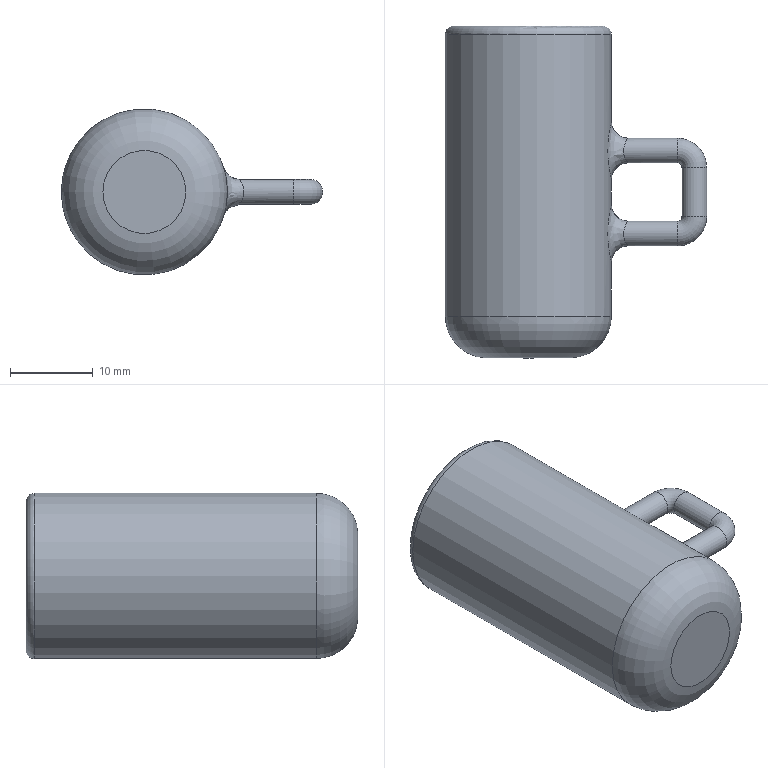Part | NX | features BLEND 4, DATUM_CSYS 2, SWP104 2, REPLACE_FACE 1, SKETCH 1, UNITE 1 | 1 solid | 16 faces | box 31.5 x 40 x 20 mm | volume 6808 mm3 | torus 6 | cylinder 5 | plane 3 | spline 2 | commonest cylinder face diameters 3 x3 14 x1 20 x1
STEP:
#1=CARTESIAN_POINT('',(-10.,5.,0.));
#2=VERTEX_POINT('',#1);
#3=CARTESIAN_POINT('',(0.,5.,0.));
#4=DIRECTION('',(0.,1.,0.));
#5=DIRECTION('',(-1.,0.,0.));
#6=AXIS2_PLACEMENT_3D('',#3,#4,#5);
#7=CIRCLE('',#6,10.);
#8=EDGE_CURVE('',#2,#2,#7,.T.);
#9=ORIENTED_EDGE('',*,*,#8,.T.);
#10=EDGE_LOOP('',(#9));
#11=FACE_BOUND('',#10,.T.);
#12=CARTESIAN_POINT('',(10.,39.,0.));
#13=VERTEX_POINT('',#12);
#14=CARTESIAN_POINT('',(0.,39.,0.));
#15=DIRECTION('',(0.,-1.,0.));
#16=DIRECTION('',(1.,0.,0.));
#17=AXIS2_PLACEMENT_3D('',#14,#15,#16);
#18=CIRCLE('',#17,10.);
#19=EDGE_CURVE('',#13,#13,#18,.T.);
#20=ORIENTED_EDGE('',*,*,#19,.T.);
#21=EDGE_LOOP('',(#20));
#22=FACE_BOUND('',#21,.T.);
#23=CARTESIAN_POINT('',(9.565,15.,2.917));
#24=VERTEX_POINT('',#23);
#25=CARTESIAN_POINT('',(9.699,12.883,2.534));
#26=CARTESIAN_POINT('',(9.475,14.998,3.173));
#27=CARTESIAN_POINT('',(9.7,17.124,2.53));
#28=CARTESIAN_POINT('',(9.942,18.269,1.264));
#29=CARTESIAN_POINT('',(10.029,18.616,0.0008688));
#30=CARTESIAN_POINT('',(9.942,18.269,-1.266));
#31=CARTESIAN_POINT('',(9.7,17.12,-2.532));
#32=CARTESIAN_POINT('',(9.475,15.,-3.173));
#33=CARTESIAN_POINT('',(9.7,12.88,-2.532));
#34=CARTESIAN_POINT('',(9.942,11.73,-1.264));
#35=CARTESIAN_POINT('',(10.029,11.384,0.005302));
#36=CARTESIAN_POINT('',(9.942,11.732,1.267));
#37=CARTESIAN_POINT('',(9.699,12.883,2.534));
#38=CARTESIAN_POINT('',(9.475,14.998,3.173));
#39=CARTESIAN_POINT('',(9.7,17.124,2.53));
#40=B_SPLINE_CURVE_WITH_KNOTS('',3,(#25,#26,#27,#28,#29,#30,#31,#32,#33,#34,#35,#36,#37,#38,#39),.UNSPECIFIED.,.T.,.F.,(1,1,1,1,1,1,1,1,1,1,1,1,1,1,1,1,1,1,1),(-0.005066,-0.003799,-0.002533,0.,0.002533,0.003799,0.005066,0.006332,0.007599,0.01013,0.01266,0.01393,0.0152,0.01646,0.01773,0.02026,0.0228,0.02406,0.02533),.UNSPECIFIED.);
#41=EDGE_CURVE('',#24,#24,#40,.T.);
#42=ORIENTED_EDGE('',*,*,#41,.T.);
#43=EDGE_LOOP('',(#42));
#44=FACE_BOUND('',#43,.T.);
#45=CARTESIAN_POINT('',(9.565,25.,2.917));
#46=VERTEX_POINT('',#45);
#47=CARTESIAN_POINT('',(9.7,22.877,2.531));
#48=CARTESIAN_POINT('',(9.475,25.,3.174));
#49=CARTESIAN_POINT('',(9.7,27.123,2.531));
#50=CARTESIAN_POINT('',(9.942,28.27,1.262));
#51=CARTESIAN_POINT('',(10.029,28.614,0.003138));
#52=CARTESIAN_POINT('',(9.943,28.272,-1.261));
#53=CARTESIAN_POINT('',(9.7,27.122,-2.532));
#54=CARTESIAN_POINT('',(9.475,25.001,-3.173));
#55=CARTESIAN_POINT('',(9.7,22.88,-2.531));
#56=CARTESIAN_POINT('',(9.942,21.732,-1.269));
#57=CARTESIAN_POINT('',(10.029,21.384,0.004067));
#58=CARTESIAN_POINT('',(9.942,21.731,1.263));
#59=CARTESIAN_POINT('',(9.7,22.877,2.531));
#60=CARTESIAN_POINT('',(9.475,25.,3.174));
#61=CARTESIAN_POINT('',(9.7,27.123,2.531));
#62=B_SPLINE_CURVE_WITH_KNOTS('',3,(#47,#48,#49,#50,#51,#52,#53,#54,#55,#56,#57,#58,#59,#60,#61),.UNSPECIFIED.,.T.,.F.,(1,1,1,1,1,1,1,1,1,1,1,1,1,1,1,1,1,1,1),(-0.005105,-0.003829,-0.002552,0.,0.002552,0.003829,0.005105,0.006381,0.007657,0.01021,0.01276,0.01404,0.01531,0.01659,0.01787,0.02042,0.02297,0.02425,0.02552),.UNSPECIFIED.);
#63=EDGE_CURVE('',#46,#46,#62,.T.);
#64=ORIENTED_EDGE('',*,*,#63,.T.);
#65=EDGE_LOOP('',(#64));
#66=FACE_BOUND('',#65,.T.);
#67=CARTESIAN_POINT('',(0.,40.,0.));
#68=DIRECTION('',(0.,-1.,0.));
#69=DIRECTION('',(1.,0.,0.));
#70=AXIS2_PLACEMENT_3D('',#67,#68,#69);
#71=CYLINDRICAL_SURFACE('',#70,10.);
#72=ADVANCED_FACE('',(#11,#22,#44,#66),#71,.T.);
#73=CARTESIAN_POINT('',(2.,2.,0.));
#74=VERTEX_POINT('',#73);
#75=CARTESIAN_POINT('',(0.,2.,0.));
#76=DIRECTION('',(0.,-1.,0.));
#77=DIRECTION('',(1.,0.,0.));
#78=AXIS2_PLACEMENT_3D('',#75,#76,#77);
#79=CIRCLE('',#78,2.);
#80=EDGE_CURVE('',#74,#74,#79,.F.);
#81=ORIENTED_EDGE('',*,*,#80,.T.);
#82=EDGE_LOOP('',(#81));
#83=FACE_BOUND('',#82,.T.);
#84=CARTESIAN_POINT('',(0.,2.,0.));
#85=DIRECTION('',(0.,-1.,0.));
#86=DIRECTION('',(1.,0.,0.));
#87=AXIS2_PLACEMENT_3D('',#84,#85,#86);
#88=PLANE('',#87);
#89=ADVANCED_FACE('',(#83),#88,.F.);
#90=CARTESIAN_POINT('',(7.,7.,0.));
#91=VERTEX_POINT('',#90);
#92=CARTESIAN_POINT('',(0.,7.,0.));
#93=DIRECTION('',(0.,-1.,0.));
#94=DIRECTION('',(1.,0.,0.));
#95=AXIS2_PLACEMENT_3D('',#92,#93,#94);
#96=CIRCLE('',#95,7.);
#97=EDGE_CURVE('',#91,#91,#96,.T.);
#98=ORIENTED_EDGE('',*,*,#97,.T.);
#99=EDGE_LOOP('',(#98));
#100=FACE_BOUND('',#99,.T.);
#101=CARTESIAN_POINT('',(7.,39.,0.));
#102=VERTEX_POINT('',#101);
#103=CARTESIAN_POINT('',(0.,39.,0.));
#104=DIRECTION('',(0.,-1.,0.));
#105=DIRECTION('',(1.,0.,0.));
#106=AXIS2_PLACEMENT_3D('',#103,#104,#105);
#107=CIRCLE('',#106,7.);
#108=EDGE_CURVE('',#102,#102,#107,.F.);
#109=ORIENTED_EDGE('',*,*,#108,.T.);
#110=EDGE_LOOP('',(#109));
#111=FACE_BOUND('',#110,.T.);
#112=CARTESIAN_POINT('',(0.,40.,0.));
#113=DIRECTION('',(0.,-1.,0.));
#114=DIRECTION('',(1.,0.,0.));
#115=AXIS2_PLACEMENT_3D('',#112,#113,#114);
#116=CYLINDRICAL_SURFACE('',#115,7.);
#117=ADVANCED_FACE('',(#100,#111),#116,.F.);
#118=CARTESIAN_POINT('',(8.,40.,0.));
#119=VERTEX_POINT('',#118);
#120=CARTESIAN_POINT('',(0.,40.,0.));
#121=DIRECTION('',(0.,-1.,0.));
#122=DIRECTION('',(1.,0.,0.));
#123=AXIS2_PLACEMENT_3D('',#120,#121,#122);
#124=CIRCLE('',#123,8.);
#125=EDGE_CURVE('',#119,#119,#124,.T.);
#126=ORIENTED_EDGE('',*,*,#125,.T.);
#127=EDGE_LOOP('',(#126));
#128=FACE_BOUND('',#127,.T.);
#129=CARTESIAN_POINT('',(9.,40.,0.));
#130=VERTEX_POINT('',#129);
#131=CARTESIAN_POINT('',(0.,40.,0.));
#132=DIRECTION('',(0.,-1.,0.));
#133=DIRECTION('',(1.,0.,0.));
#134=AXIS2_PLACEMENT_3D('',#131,#132,#133);
#135=CIRCLE('',#134,9.);
#136=EDGE_CURVE('',#130,#130,#135,.F.);
#137=ORIENTED_EDGE('',*,*,#136,.T.);
#138=EDGE_LOOP('',(#137));
#139=FACE_BOUND('',#138,.T.);
#140=CARTESIAN_POINT('',(7.,40.,0.));
#141=DIRECTION('',(0.,-1.,0.));
#142=DIRECTION('',(1.,0.,0.));
#143=AXIS2_PLACEMENT_3D('',#140,#141,#142);
#144=PLANE('',#143);
#145=ADVANCED_FACE('',(#128,#139),#144,.F.);
#146=CARTESIAN_POINT('',(-5.,0.,0.));
#147=VERTEX_POINT('',#146);
#148=CARTESIAN_POINT('',(0.,0.,0.));
#149=DIRECTION('',(0.,1.,0.));
#150=DIRECTION('',(-1.,0.,0.));
#151=AXIS2_PLACEMENT_3D('',#148,#149,#150);
#152=CIRCLE('',#151,5.);
#153=EDGE_CURVE('',#147,#147,#152,.F.);
#154=ORIENTED_EDGE('',*,*,#153,.T.);
#155=EDGE_LOOP('',(#154));
#156=FACE_BOUND('',#155,.T.);
#157=CARTESIAN_POINT('',(10.,0.,0.));
#158=DIRECTION('',(0.,1.,0.));
#159=DIRECTION('',(-1.,0.,0.));
#160=AXIS2_PLACEMENT_3D('',#157,#158,#159);
#161=PLANE('',#160);
#162=ADVANCED_FACE('',(#156),#161,.F.);
#163=CARTESIAN_POINT('',(11.478,25.,1.5));
#164=VERTEX_POINT('',#163);
#165=CARTESIAN_POINT('',(11.745,26.176,1.174));
#166=CARTESIAN_POINT('',(11.345,25.,1.663));
#167=CARTESIAN_POINT('',(11.745,23.824,1.175));
#168=CARTESIAN_POINT('',(12.128,23.337,-0.001731));
#169=CARTESIAN_POINT('',(11.744,23.827,-1.177));
#170=CARTESIAN_POINT('',(11.345,24.999,-1.662));
#171=CARTESIAN_POINT('',(11.745,26.176,-1.176));
#172=CARTESIAN_POINT('',(12.127,26.662,0.0008474));
#173=CARTESIAN_POINT('',(11.745,26.176,1.174));
#174=CARTESIAN_POINT('',(11.345,25.,1.663));
#175=CARTESIAN_POINT('',(11.745,23.824,1.175));
#176=B_SPLINE_CURVE_WITH_KNOTS('',3,(#165,#166,#167,#168,#169,#170,#171,#172,#173,#174,#175),.UNSPECIFIED.,.T.,.F.,(1,1,1,1,1,1,1,1,1,1,1,1,1,1,1),(-0.003636,-0.002424,-0.001212,0.,0.001212,0.002424,0.003636,0.004848,0.006061,0.007273,0.008485,0.009697,0.01091,0.01212,0.01333),.UNSPECIFIED.);
#177=EDGE_CURVE('',#164,#164,#176,.T.);
#178=ORIENTED_EDGE('',*,*,#177,.T.);
#179=EDGE_LOOP('',(#178));
#180=FACE_BOUND('',#179,.T.);
#181=CARTESIAN_POINT('',(18.,25.,-1.5));
#182=VERTEX_POINT('',#181);
#183=CARTESIAN_POINT('',(18.,25.,0.));
#184=DIRECTION('',(-1.,0.,0.));
#185=DIRECTION('',(0.,0.,-1.));
#186=AXIS2_PLACEMENT_3D('',#183,#184,#185);
#187=CIRCLE('',#186,1.5);
#188=EDGE_CURVE('',#182,#182,#187,.T.);
#189=ORIENTED_EDGE('',*,*,#188,.T.);
#190=EDGE_LOOP('',(#189));
#191=FACE_BOUND('',#190,.T.);
#192=CARTESIAN_POINT('',(18.,25.,0.));
#193=DIRECTION('',(-1.,0.,0.));
#194=DIRECTION('',(0.,0.,1.));
#195=AXIS2_PLACEMENT_3D('',#192,#193,#194);
#196=CYLINDRICAL_SURFACE('',#195,1.5);
#197=ADVANCED_FACE('',(#180,#191),#196,.T.);
#198=CARTESIAN_POINT('',(20.,23.,-1.5));
#199=VERTEX_POINT('',#198);
#200=CARTESIAN_POINT('',(20.,23.,0.));
#201=DIRECTION('',(0.,1.,0.));
#202=DIRECTION('',(0.,0.,-1.));
#203=AXIS2_PLACEMENT_3D('',#200,#201,#202);
#204=CIRCLE('',#203,1.5);
#205=EDGE_CURVE('',#199,#199,#204,.T.);
#206=ORIENTED_EDGE('',*,*,#205,.T.);
#207=EDGE_LOOP('',(#206));
#208=FACE_BOUND('',#207,.T.);
#209=ORIENTED_EDGE('',*,*,#188,.F.);
#210=EDGE_LOOP('',(#209));
#211=FACE_BOUND('',#210,.T.);
#212=CARTESIAN_POINT('',(18.,23.,0.));
#213=DIRECTION('',(0.,0.,1.));
#214=DIRECTION('',(1.,0.,0.));
#215=AXIS2_PLACEMENT_3D('',#212,#213,#214);
#216=TOROIDAL_SURFACE('',#215,2.,1.5);
#217=ADVANCED_FACE('',(#208,#211),#216,.T.);
#218=CARTESIAN_POINT('',(20.,17.,-1.5));
#219=VERTEX_POINT('',#218);
#220=CARTESIAN_POINT('',(20.,17.,0.));
#221=DIRECTION('',(0.,1.,0.));
#222=DIRECTION('',(0.,0.,-1.));
#223=AXIS2_PLACEMENT_3D('',#220,#221,#222);
#224=CIRCLE('',#223,1.5);
#225=EDGE_CURVE('',#219,#219,#224,.T.);
#226=ORIENTED_EDGE('',*,*,#225,.T.);
#227=EDGE_LOOP('',(#226));
#228=FACE_BOUND('',#227,.T.);
#229=ORIENTED_EDGE('',*,*,#205,.F.);
#230=EDGE_LOOP('',(#229));
#231=FACE_BOUND('',#230,.T.);
#232=CARTESIAN_POINT('',(20.,17.,0.));
#233=DIRECTION('',(0.,1.,0.));
#234=DIRECTION('',(0.,0.,1.));
#235=AXIS2_PLACEMENT_3D('',#232,#233,#234);
#236=CYLINDRICAL_SURFACE('',#235,1.5);
#237=ADVANCED_FACE('',(#228,#231),#236,.T.);
#238=CARTESIAN_POINT('',(18.,15.,-1.5));
#239=VERTEX_POINT('',#238);
#240=CARTESIAN_POINT('',(18.,15.,0.));
#241=DIRECTION('',(1.,0.,0.));
#242=DIRECTION('',(0.,0.,-1.));
#243=AXIS2_PLACEMENT_3D('',#240,#241,#242);
#244=CIRCLE('',#243,1.5);
#245=EDGE_CURVE('',#239,#239,#244,.T.);
#246=ORIENTED_EDGE('',*,*,#245,.T.);
#247=EDGE_LOOP('',(#246));
#248=FACE_BOUND('',#247,.T.);
#249=ORIENTED_EDGE('',*,*,#225,.F.);
#250=EDGE_LOOP('',(#249));
#251=FACE_BOUND('',#250,.T.);
#252=CARTESIAN_POINT('',(18.,17.,0.));
#253=DIRECTION('',(0.,0.,1.));
#254=DIRECTION('',(1.,0.,0.));
#255=AXIS2_PLACEMENT_3D('',#252,#253,#254);
#256=TOROIDAL_SURFACE('',#255,2.,1.5);
#257=ADVANCED_FACE('',(#248,#251),#256,.T.);
#258=CARTESIAN_POINT('',(11.478,15.,1.5));
#259=VERTEX_POINT('',#258);
#260=CARTESIAN_POINT('',(11.745,16.175,1.175));
#261=CARTESIAN_POINT('',(11.345,15.,1.663));
#262=CARTESIAN_POINT('',(11.746,13.823,1.174));
#263=CARTESIAN_POINT('',(12.128,13.338,-0.001501));
#264=CARTESIAN_POINT('',(11.744,13.826,-1.177));
#265=CARTESIAN_POINT('',(11.345,15.002,-1.662));
#266=CARTESIAN_POINT('',(11.745,16.175,-1.176));
#267=CARTESIAN_POINT('',(12.128,16.663,0.002663));
#268=CARTESIAN_POINT('',(11.745,16.175,1.175));
#269=CARTESIAN_POINT('',(11.345,15.,1.663));
#270=CARTESIAN_POINT('',(11.746,13.823,1.174));
#271=B_SPLINE_CURVE_WITH_KNOTS('',3,(#260,#261,#262,#263,#264,#265,#266,#267,#268,#269,#270),.UNSPECIFIED.,.T.,.F.,(1,1,1,1,1,1,1,1,1,1,1,1,1,1,1),(-0.003683,-0.002456,-0.001228,0.,0.001228,0.002456,0.003683,0.004911,0.006139,0.007367,0.008595,0.009822,0.01105,0.01228,0.01351),.UNSPECIFIED.);
#272=EDGE_CURVE('',#259,#259,#271,.T.);
#273=ORIENTED_EDGE('',*,*,#272,.T.);
#274=EDGE_LOOP('',(#273));
#275=FACE_BOUND('',#274,.T.);
#276=ORIENTED_EDGE('',*,*,#245,.F.);
#277=EDGE_LOOP('',(#276));
#278=FACE_BOUND('',#277,.T.);
#279=CARTESIAN_POINT('',(18.,15.,0.));
#280=DIRECTION('',(-1.,0.,0.));
#281=DIRECTION('',(0.,0.,1.));
#282=AXIS2_PLACEMENT_3D('',#279,#280,#281);
#283=CYLINDRICAL_SURFACE('',#282,1.5);
#284=ADVANCED_FACE('',(#275,#278),#283,.T.);
#285=ORIENTED_EDGE('',*,*,#41,.F.);
#286=EDGE_LOOP('',(#285));
#287=FACE_BOUND('',#286,.T.);
#288=ORIENTED_EDGE('',*,*,#272,.F.);
#289=EDGE_LOOP('',(#288));
#290=FACE_BOUND('',#289,.T.);
#291=CARTESIAN_POINT('',(9.566,14.895,2.915));
#292=CARTESIAN_POINT('',(9.997,14.941,1.499));
#293=CARTESIAN_POINT('',(11.479,14.955,1.499));
#294=CARTESIAN_POINT('',(9.559,15.808,2.938));
#295=CARTESIAN_POINT('',(9.996,15.423,1.515));
#296=CARTESIAN_POINT('',(11.471,15.346,1.511));
#297=CARTESIAN_POINT('',(9.712,17.197,2.493));
#298=CARTESIAN_POINT('',(10.047,16.225,1.087));
#299=CARTESIAN_POINT('',(11.654,15.942,1.282));
#300=CARTESIAN_POINT('',(9.943,18.271,1.233));
#301=CARTESIAN_POINT('',(10.023,16.484,0.3943));
#302=CARTESIAN_POINT('',(11.932,16.402,0.6339));
#303=CARTESIAN_POINT('',(10.023,18.591,0.09203));
#304=CARTESIAN_POINT('',(9.99,16.506,0.02435));
#305=CARTESIAN_POINT('',(12.027,16.539,0.04733));
#306=CARTESIAN_POINT('',(9.964,18.355,-1.067));
#307=CARTESIAN_POINT('',(10.016,16.493,-0.3266));
#308=CARTESIAN_POINT('',(11.956,16.438,-0.5486));
#309=CARTESIAN_POINT('',(9.743,17.367,-2.383));
#310=CARTESIAN_POINT('',(10.052,16.292,-0.9981));
#311=CARTESIAN_POINT('',(11.692,16.014,-1.226));
#312=CARTESIAN_POINT('',(9.458,15.118,-3.233));
#313=CARTESIAN_POINT('',(9.965,15.077,-1.783));
#314=CARTESIAN_POINT('',(11.349,15.051,-1.663));
#315=CARTESIAN_POINT('',(9.712,12.803,-2.494));
#316=CARTESIAN_POINT('',(10.047,13.775,-1.088));
#317=CARTESIAN_POINT('',(11.654,14.059,-1.283));
#318=CARTESIAN_POINT('',(9.944,11.728,-1.231));
#319=CARTESIAN_POINT('',(10.023,13.516,-0.3934));
#320=CARTESIAN_POINT('',(11.933,13.598,-0.6329));
#321=CARTESIAN_POINT('',(10.023,11.409,-0.08913));
#322=CARTESIAN_POINT('',(9.99,13.494,-0.02362));
#323=CARTESIAN_POINT('',(12.027,13.461,-0.04584));
#324=CARTESIAN_POINT('',(9.963,11.646,1.068));
#325=CARTESIAN_POINT('',(10.016,13.507,0.3273));
#326=CARTESIAN_POINT('',(11.956,13.563,0.5493));
#327=CARTESIAN_POINT('',(9.744,12.631,2.382));
#328=CARTESIAN_POINT('',(10.052,13.708,0.9973));
#329=CARTESIAN_POINT('',(11.692,13.985,1.225));
#330=CARTESIAN_POINT('',(9.572,13.982,2.893));
#331=CARTESIAN_POINT('',(9.998,14.458,1.482));
#332=CARTESIAN_POINT('',(11.486,14.564,1.488));
#333=CARTESIAN_POINT('',(9.566,14.895,2.915));
#334=CARTESIAN_POINT('',(9.997,14.941,1.499));
#335=CARTESIAN_POINT('',(11.479,14.955,1.499));
#336=(BOUNDED_SURFACE()B_SPLINE_SURFACE(3,2,((#291,#292,#293),(#294,#295,#296),(#297,#298,#299),(#300,#301,#302),(#303,#304,#305),(#306,#307,#308),(#309,#310,#311),(#312,#313,#314),(#315,#316,#317),(#318,#319,#320),(#321,#322,#323),(#324,#325,#326),(#327,#328,#329),(#330,#331,#332),(#333,#334,#335)),.UNSPECIFIED.,.T.,.F.,.F.)B_SPLINE_SURFACE_WITH_KNOTS((1,3,1,1,1,1,1,1,1,1,1,1,1,3,1),(3,3),(-0.002751,0.,0.002751,0.004126,0.005502,0.006877,0.008252,0.011,0.01375,0.01513,0.0165,0.01788,0.01926,0.02201,0.02476),(0.,1.),.UNSPECIFIED.)GEOMETRIC_REPRESENTATION_ITEM()RATIONAL_B_SPLINE_SURFACE(((1.,0.8036,1.),(1.,0.8049,1.),(1.,0.774,1.),(1.,0.721,1.),(1.,0.7015,1.),(1.,0.7161,1.),(1.,0.7673,1.),(1.,0.8255,1.),(1.,0.774,1.),(1.,0.7209,1.),(1.,0.7015,1.),(1.,0.7161,1.),(1.,0.7672,1.),(1.,0.8022,1.),(1.,0.8036,1.)))REPRESENTATION_ITEM('')SURFACE());
#337=ADVANCED_FACE('',(#287,#290),#336,.F.);
#338=ORIENTED_EDGE('',*,*,#177,.F.);
#339=EDGE_LOOP('',(#338));
#340=FACE_BOUND('',#339,.T.);
#341=ORIENTED_EDGE('',*,*,#63,.F.);
#342=EDGE_LOOP('',(#341));
#343=FACE_BOUND('',#342,.T.);
#344=CARTESIAN_POINT('',(9.595,24.089,2.816));
#345=CARTESIAN_POINT('',(10.006,24.498,1.418));
#346=CARTESIAN_POINT('',(11.514,24.61,1.448));
#347=CARTESIAN_POINT('',(9.566,24.532,2.916));
#348=CARTESIAN_POINT('',(9.998,24.734,1.497));
#349=CARTESIAN_POINT('',(11.479,24.8,1.499));
#350=CARTESIAN_POINT('',(9.549,25.472,2.968));
#351=CARTESIAN_POINT('',(9.992,25.273,1.543));
#352=CARTESIAN_POINT('',(11.459,25.202,1.526));
#353=CARTESIAN_POINT('',(9.665,26.8,2.589));
#354=CARTESIAN_POINT('',(10.027,25.989,1.223));
#355=CARTESIAN_POINT('',(11.598,25.771,1.331));
#356=CARTESIAN_POINT('',(9.847,27.844,1.825));
#357=CARTESIAN_POINT('',(10.041,26.399,0.6952));
#358=CARTESIAN_POINT('',(11.816,26.219,0.9385));
#359=CARTESIAN_POINT('',(9.991,28.467,0.7827));
#360=CARTESIAN_POINT('',(10.005,26.504,0.2247));
#361=CARTESIAN_POINT('',(11.989,26.486,0.4025));
#362=CARTESIAN_POINT('',(10.015,28.562,-0.3904));
#363=CARTESIAN_POINT('',(9.994,26.505,-0.1049));
#364=CARTESIAN_POINT('',(12.018,26.527,-0.2008));
#365=CARTESIAN_POINT('',(9.904,28.107,-1.5));
#366=CARTESIAN_POINT('',(10.033,26.461,-0.5193));
#367=CARTESIAN_POINT('',(11.885,26.331,-0.7716));
#368=CARTESIAN_POINT('',(9.724,27.189,-2.371));
#369=CARTESIAN_POINT('',(10.037,26.165,-1.057));
#370=CARTESIAN_POINT('',(11.668,25.938,-1.219));
#371=CARTESIAN_POINT('',(9.575,25.938,-2.889));
#372=CARTESIAN_POINT('',(10.001,25.537,-1.474));
#373=CARTESIAN_POINT('',(11.49,25.402,-1.486));
#374=CARTESIAN_POINT('',(9.549,24.53,-2.968));
#375=CARTESIAN_POINT('',(9.992,24.727,-1.543));
#376=CARTESIAN_POINT('',(11.459,24.798,-1.526));
#377=CARTESIAN_POINT('',(9.665,23.201,-2.589));
#378=CARTESIAN_POINT('',(10.027,24.011,-1.224));
#379=CARTESIAN_POINT('',(11.598,24.229,-1.332));
#380=CARTESIAN_POINT('',(9.847,22.154,-1.823));
#381=CARTESIAN_POINT('',(10.041,23.6,-0.694));
#382=CARTESIAN_POINT('',(11.817,23.78,-0.9376));
#383=CARTESIAN_POINT('',(9.991,21.532,-0.7798));
#384=CARTESIAN_POINT('',(10.005,23.496,-0.2238));
#385=CARTESIAN_POINT('',(11.989,23.514,-0.401));
#386=CARTESIAN_POINT('',(10.015,21.439,0.3926));
#387=CARTESIAN_POINT('',(9.994,23.495,0.1056));
#388=CARTESIAN_POINT('',(12.018,23.474,0.2019));
#389=CARTESIAN_POINT('',(9.904,21.893,1.499));
#390=CARTESIAN_POINT('',(10.033,23.539,0.5189));
#391=CARTESIAN_POINT('',(11.885,23.668,0.7711));
#392=CARTESIAN_POINT('',(9.724,22.811,2.371));
#393=CARTESIAN_POINT('',(10.037,23.834,1.056));
#394=CARTESIAN_POINT('',(11.669,24.062,1.219));
#395=CARTESIAN_POINT('',(9.624,23.645,2.717));
#396=CARTESIAN_POINT('',(10.013,24.259,1.338));
#397=CARTESIAN_POINT('',(11.549,24.419,1.397));
#398=CARTESIAN_POINT('',(9.595,24.089,2.816));
#399=CARTESIAN_POINT('',(10.006,24.498,1.418));
#400=CARTESIAN_POINT('',(11.514,24.61,1.448));
#401=(BOUNDED_SURFACE()B_SPLINE_SURFACE(3,2,((#344,#345,#346),(#347,#348,#349),(#350,#351,#352),(#353,#354,#355),(#356,#357,#358),(#359,#360,#361),(#362,#363,#364),(#365,#366,#367),(#368,#369,#370),(#371,#372,#373),(#374,#375,#376),(#377,#378,#379),(#380,#381,#382),(#383,#384,#385),(#386,#387,#388),(#389,#390,#391),(#392,#393,#394),(#395,#396,#397),(#398,#399,#400)),.UNSPECIFIED.,.T.,.F.,.F.)B_SPLINE_SURFACE_WITH_KNOTS((1,3,1,1,1,1,1,1,1,1,1,1,1,1,1,1,1,3,1),(3,3),(-0.001374,0.,0.001374,0.002748,0.004122,0.005497,0.006871,0.008245,0.009619,0.01099,0.01237,0.01374,0.01512,0.01649,0.01786,0.01924,0.02061,0.02199,0.02336),(0.,1.),.UNSPECIFIED.)GEOMETRIC_REPRESENTATION_ITEM()RATIONAL_B_SPLINE_SURFACE(((1.,0.7975,1.),(1.,0.8035,1.),(1.,0.8069,1.),(1.,0.7832,1.),(1.,0.7435,1.),(1.,0.7094,1.),(1.,0.7034,1.),(1.,0.7302,1.),(1.,0.7708,1.),(1.,0.8018,1.),(1.,0.8069,1.),(1.,0.7833,1.),(1.,0.7434,1.),(1.,0.7093,1.),(1.,0.7034,1.),(1.,0.7302,1.),(1.,0.7708,1.),(1.,0.7915,1.),(1.,0.7975,1.)))REPRESENTATION_ITEM('')SURFACE());
#402=ADVANCED_FACE('',(#340,#343),#401,.F.);
#403=ORIENTED_EDGE('',*,*,#108,.F.);
#404=EDGE_LOOP('',(#403));
#405=FACE_BOUND('',#404,.T.);
#406=ORIENTED_EDGE('',*,*,#125,.F.);
#407=EDGE_LOOP('',(#406));
#408=FACE_BOUND('',#407,.T.);
#409=CARTESIAN_POINT('',(0.,39.,0.));
#410=DIRECTION('',(0.,-1.,0.));
#411=DIRECTION('',(1.,0.,0.));
#412=AXIS2_PLACEMENT_3D('',#409,#410,#411);
#413=TOROIDAL_SURFACE('',#412,8.,1.);
#414=ADVANCED_FACE('',(#405,#408),#413,.T.);
#415=ORIENTED_EDGE('',*,*,#136,.F.);
#416=EDGE_LOOP('',(#415));
#417=FACE_BOUND('',#416,.T.);
#418=ORIENTED_EDGE('',*,*,#19,.F.);
#419=EDGE_LOOP('',(#418));
#420=FACE_BOUND('',#419,.T.);
#421=CARTESIAN_POINT('',(0.,39.,0.));
#422=DIRECTION('',(0.,-1.,0.));
#423=DIRECTION('',(1.,0.,0.));
#424=AXIS2_PLACEMENT_3D('',#421,#422,#423);
#425=TOROIDAL_SURFACE('',#424,9.,1.);
#426=ADVANCED_FACE('',(#417,#420),#425,.T.);
#427=ORIENTED_EDGE('',*,*,#8,.F.);
#428=EDGE_LOOP('',(#427));
#429=FACE_BOUND('',#428,.T.);
#430=ORIENTED_EDGE('',*,*,#153,.F.);
#431=EDGE_LOOP('',(#430));
#432=FACE_BOUND('',#431,.T.);
#433=CARTESIAN_POINT('',(0.,5.,0.));
#434=DIRECTION('',(0.,1.,0.));
#435=DIRECTION('',(-1.,0.,0.));
#436=AXIS2_PLACEMENT_3D('',#433,#434,#435);
#437=TOROIDAL_SURFACE('',#436,5.,5.);
#438=ADVANCED_FACE('',(#429,#432),#437,.T.);
#439=ORIENTED_EDGE('',*,*,#80,.F.);
#440=EDGE_LOOP('',(#439));
#441=FACE_BOUND('',#440,.T.);
#442=ORIENTED_EDGE('',*,*,#97,.F.);
#443=EDGE_LOOP('',(#442));
#444=FACE_BOUND('',#443,.T.);
#445=CARTESIAN_POINT('',(0.,7.,0.));
#446=DIRECTION('',(0.,-1.,0.));
#447=DIRECTION('',(1.,0.,0.));
#448=AXIS2_PLACEMENT_3D('',#445,#446,#447);
#449=DEGENERATE_TOROIDAL_SURFACE('',#448,2.,5.,.T.);
#450=ADVANCED_FACE('',(#441,#444),#449,.F.);
#451=CLOSED_SHELL('',(#72,#89,#117,#145,#162,#197,#217,#237,#257,#284,#337,#402,#414,#426,#438,#450));
#452=MANIFOLD_SOLID_BREP('',#451);
#453=(LENGTH_UNIT()NAMED_UNIT(*)SI_UNIT(.MILLI.,.METRE.));
#454=UNCERTAINTY_MEASURE_WITH_UNIT(LENGTH_MEASURE(0.0508),#453,'','');
#455=(NAMED_UNIT(*)PLANE_ANGLE_UNIT()SI_UNIT($,.RADIAN.));
#456=(NAMED_UNIT(*)SI_UNIT($,.STERADIAN.)SOLID_ANGLE_UNIT());
#457=(GEOMETRIC_REPRESENTATION_CONTEXT(3)GLOBAL_UNCERTAINTY_ASSIGNED_CONTEXT((#454))GLOBAL_UNIT_ASSIGNED_CONTEXT((#453,#455,#456))REPRESENTATION_CONTEXT('',''));
#458=ADVANCED_BREP_SHAPE_REPRESENTATION('',(#452),#457);